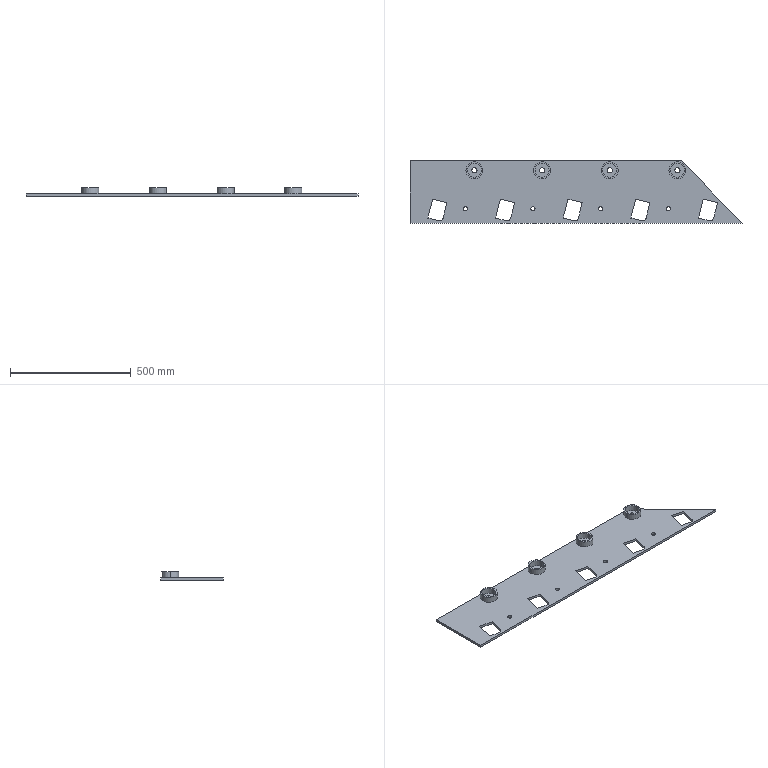Part | STEP file | Edge plate 5_Default<As machined> | 5 solids | 71 faces | box 1374 x 260 x 35 mm | volume 3099117 mm3 | cylinder 37 | plane 34 | commonest cylinder face diameters 17 x8 22 x8 58 x8 70 x8 30 x5